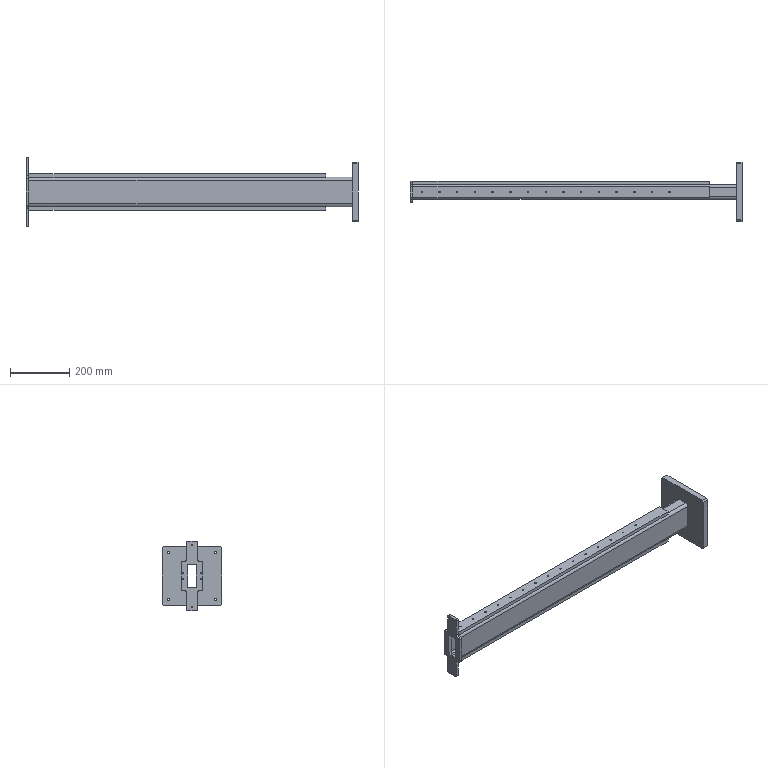Part | SolidWorks | features ICE 7, HoleWzd 5, Chamfer 2, Fillet 2, Cut 1, EndCap 1, MirrorPattern 1, MoveFace 1, WeldMemberFeat 1, WeldmentFeature 1 | 6 solids | 298 faces | box 1125 x 200 x 236 mm | volume 3630332 mm3 | cylinder 172 | plane 66 | cone 60 | commonest cylinder face diameters 5 x124 10 x20 2.5 x8 4.2 x8 8.5 x8 20 x4